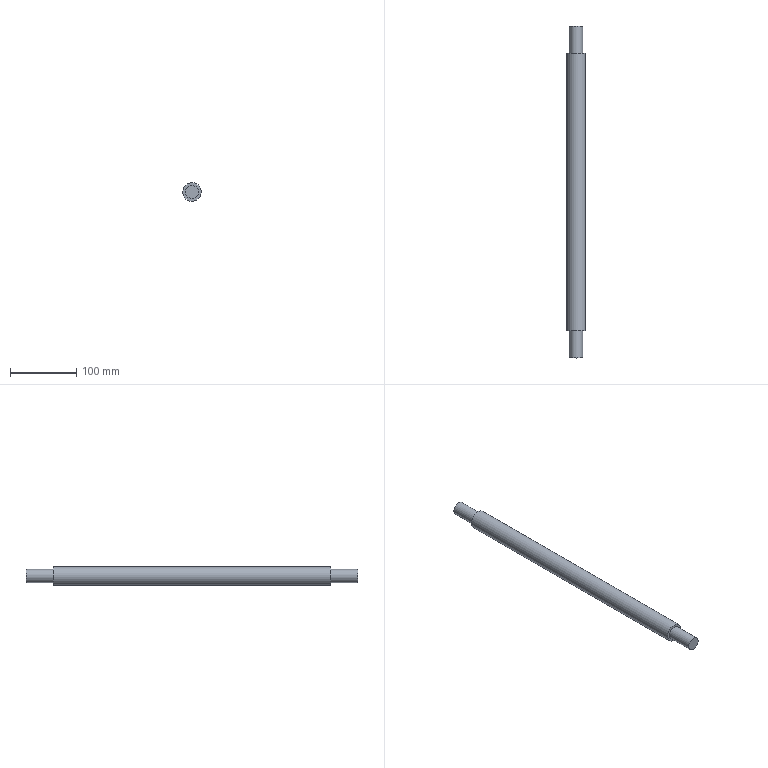Part | STEP file | SN10_002_010-03_EIXO | 1 solid | 7 faces | box 28 x 500.1 x 28 mm | volume 283207 mm3 | plane 4 | cylinder 3 | commonest cylinder face diameters 20 x2 28 x1
STEP:
#1=CARTESIAN_POINT('',(0.,0.,0.));
#2=DIRECTION('',(0.,0.,1.));
#3=DIRECTION('',(1.,0.,0.));
#4=AXIS2_PLACEMENT_3D('',#1,#2,#3);
#5=CARTESIAN_POINT('',(995.206,90.05,8.776));
#6=VERTEX_POINT('',#5);
#7=CARTESIAN_POINT('',(1000.,90.05,0.));
#8=DIRECTION('',(0.,-1.,0.));
#9=DIRECTION('',(1.,0.,0.));
#10=AXIS2_PLACEMENT_3D('',#7,#8,#9);
#11=CIRCLE('',#10,10.);
#12=CARTESIAN_POINT('',(1000.,-160.,0.));
#13=DIRECTION('',(0.,-1.,0.));
#14=DIRECTION('',(-0.4794,0.,0.8776));
#15=AXIS2_PLACEMENT_3D('',#12,#13,#14);
#16=CYLINDRICAL_SURFACE('',#15,10.);
#17=CARTESIAN_POINT('',(-2.071,-250.05));
#18=DIRECTION('',(1.,0.));
#19=VECTOR('',#18,1.);
#20=LINE('',#17,#19);
#21=(GEOMETRIC_REPRESENTATION_CONTEXT(2)PARAMETRIC_REPRESENTATION_CONTEXT()REPRESENTATION_CONTEXT('',''));
#22=DEFINITIONAL_REPRESENTATION('',(#20),#21);
#23=PCURVE('',#16,#22);
#24=CARTESIAN_POINT('',(1000.,90.05,10.));
#25=DIRECTION('',(0.,-1.,0.));
#26=DIRECTION('',(0.,0.,-1.));
#27=AXIS2_PLACEMENT_3D('',#24,#25,#26);
#28=PLANE('',#27);
#29=CARTESIAN_POINT('',(10.,0.));
#30=DIRECTION('',(0.,1.));
#31=AXIS2_PLACEMENT_2D('',#29,#30);
#32=CIRCLE('',#31,10.);
#33=(GEOMETRIC_REPRESENTATION_CONTEXT(2)PARAMETRIC_REPRESENTATION_CONTEXT()REPRESENTATION_CONTEXT('',''));
#34=DEFINITIONAL_REPRESENTATION('',(#32),#33);
#35=PCURVE('',#28,#34);
#36=SURFACE_CURVE('',#11,(#23,#35),.PCURVE_S1.);
#37=EDGE_CURVE('',#6,#6,#36,.T.);
#38=ORIENTED_EDGE('',*,*,#37,.T.);
#39=CARTESIAN_POINT('',(995.206,49.05,8.776));
#40=VERTEX_POINT('',#39);
#41=CARTESIAN_POINT('',(995.206,90.05,8.776));
#42=CARTESIAN_POINT('',(995.206,49.05,8.776));
#43=B_SPLINE_CURVE_WITH_KNOTS('',1,(#41,#42),.UNSPECIFIED.,.F.,.F.,(2,2),(-250.05,-209.05),.PIECEWISE_BEZIER_KNOTS.);
#44=CARTESIAN_POINT('',(6.283,0.));
#45=DIRECTION('',(0.,1.));
#46=VECTOR('',#45,1.);
#47=LINE('',#44,#46);
#48=(GEOMETRIC_REPRESENTATION_CONTEXT(2)PARAMETRIC_REPRESENTATION_CONTEXT()REPRESENTATION_CONTEXT('',''));
#49=DEFINITIONAL_REPRESENTATION('',(#47),#48);
#50=PCURVE('',#16,#49);
#51=CARTESIAN_POINT('',(0.,0.));
#52=DIRECTION('',(0.,1.));
#53=VECTOR('',#52,1.);
#54=LINE('',#51,#53);
#55=(GEOMETRIC_REPRESENTATION_CONTEXT(2)PARAMETRIC_REPRESENTATION_CONTEXT()REPRESENTATION_CONTEXT('',''));
#56=DEFINITIONAL_REPRESENTATION('',(#54),#55);
#57=PCURVE('',#16,#56);
#58=SEAM_CURVE('',#43,(#50,#57),.PCURVE_S1.);
#59=EDGE_CURVE('',#6,#40,#58,.T.);
#60=ORIENTED_EDGE('',*,*,#59,.T.);
#61=CARTESIAN_POINT('',(1000.,49.05,0.));
#62=DIRECTION('',(0.,-1.,0.));
#63=DIRECTION('',(1.,0.,0.));
#64=AXIS2_PLACEMENT_3D('',#61,#62,#63);
#65=CIRCLE('',#64,10.);
#66=CARTESIAN_POINT('',(-2.071,-209.05));
#67=DIRECTION('',(1.,0.));
#68=VECTOR('',#67,1.);
#69=LINE('',#66,#68);
#70=(GEOMETRIC_REPRESENTATION_CONTEXT(2)PARAMETRIC_REPRESENTATION_CONTEXT()REPRESENTATION_CONTEXT('',''));
#71=DEFINITIONAL_REPRESENTATION('',(#69),#70);
#72=PCURVE('',#16,#71);
#73=CARTESIAN_POINT('',(1000.,49.05,14.));
#74=DIRECTION('',(0.,-1.,0.));
#75=DIRECTION('',(0.,0.,-1.));
#76=AXIS2_PLACEMENT_3D('',#73,#74,#75);
#77=PLANE('',#76);
#78=CARTESIAN_POINT('',(14.,0.));
#79=DIRECTION('',(0.,1.));
#80=AXIS2_PLACEMENT_2D('',#78,#79);
#81=CIRCLE('',#80,10.);
#82=(GEOMETRIC_REPRESENTATION_CONTEXT(2)PARAMETRIC_REPRESENTATION_CONTEXT()REPRESENTATION_CONTEXT('',''));
#83=DEFINITIONAL_REPRESENTATION('',(#81),#82);
#84=PCURVE('',#77,#83);
#85=SURFACE_CURVE('',#65,(#72,#84),.PCURVE_S1.);
#86=EDGE_CURVE('',#40,#40,#85,.T.);
#87=ORIENTED_EDGE('',*,*,#86,.F.);
#88=ORIENTED_EDGE('',*,*,#59,.F.);
#89=EDGE_LOOP('',(#38,#60,#87,#88));
#90=FACE_BOUND('',#89,.T.);
#91=ADVANCED_FACE('',(#90),#16,.T.);
#92=CARTESIAN_POINT('',(993.288,49.05,12.286));
#93=VERTEX_POINT('',#92);
#94=CARTESIAN_POINT('',(1000.,49.05,0.));
#95=DIRECTION('',(0.,-1.,0.));
#96=DIRECTION('',(1.,0.,0.));
#97=AXIS2_PLACEMENT_3D('',#94,#95,#96);
#98=CIRCLE('',#97,14.);
#99=CARTESIAN_POINT('',(1000.,-160.,0.));
#100=DIRECTION('',(0.,-1.,0.));
#101=DIRECTION('',(-0.4794,0.,0.8776));
#102=AXIS2_PLACEMENT_3D('',#99,#100,#101);
#103=CYLINDRICAL_SURFACE('',#102,14.);
#104=CARTESIAN_POINT('',(-2.071,-209.05));
#105=DIRECTION('',(1.,0.));
#106=VECTOR('',#105,1.);
#107=LINE('',#104,#106);
#108=(GEOMETRIC_REPRESENTATION_CONTEXT(2)PARAMETRIC_REPRESENTATION_CONTEXT()REPRESENTATION_CONTEXT('',''));
#109=DEFINITIONAL_REPRESENTATION('',(#107),#108);
#110=PCURVE('',#103,#109);
#111=CARTESIAN_POINT('',(14.,0.));
#112=DIRECTION('',(0.,1.));
#113=AXIS2_PLACEMENT_2D('',#111,#112);
#114=CIRCLE('',#113,14.);
#115=(GEOMETRIC_REPRESENTATION_CONTEXT(2)PARAMETRIC_REPRESENTATION_CONTEXT()REPRESENTATION_CONTEXT('',''));
#116=DEFINITIONAL_REPRESENTATION('',(#114),#115);
#117=PCURVE('',#77,#116);
#118=SURFACE_CURVE('',#98,(#110,#117),.PCURVE_S1.);
#119=EDGE_CURVE('',#93,#93,#118,.T.);
#120=ORIENTED_EDGE('',*,*,#119,.T.);
#121=CARTESIAN_POINT('',(993.288,-369.05,12.286));
#122=VERTEX_POINT('',#121);
#123=CARTESIAN_POINT('',(993.288,49.05,12.286));
#124=CARTESIAN_POINT('',(993.288,-369.05,12.286));
#125=B_SPLINE_CURVE_WITH_KNOTS('',1,(#123,#124),.UNSPECIFIED.,.F.,.F.,(2,2),(-209.05,209.05),.PIECEWISE_BEZIER_KNOTS.);
#126=CARTESIAN_POINT('',(6.283,0.));
#127=DIRECTION('',(0.,1.));
#128=VECTOR('',#127,1.);
#129=LINE('',#126,#128);
#130=(GEOMETRIC_REPRESENTATION_CONTEXT(2)PARAMETRIC_REPRESENTATION_CONTEXT()REPRESENTATION_CONTEXT('',''));
#131=DEFINITIONAL_REPRESENTATION('',(#129),#130);
#132=PCURVE('',#103,#131);
#133=CARTESIAN_POINT('',(0.,0.));
#134=DIRECTION('',(0.,1.));
#135=VECTOR('',#134,1.);
#136=LINE('',#133,#135);
#137=(GEOMETRIC_REPRESENTATION_CONTEXT(2)PARAMETRIC_REPRESENTATION_CONTEXT()REPRESENTATION_CONTEXT('',''));
#138=DEFINITIONAL_REPRESENTATION('',(#136),#137);
#139=PCURVE('',#103,#138);
#140=SEAM_CURVE('',#125,(#132,#139),.PCURVE_S1.);
#141=EDGE_CURVE('',#93,#122,#140,.T.);
#142=ORIENTED_EDGE('',*,*,#141,.T.);
#143=CARTESIAN_POINT('',(1000.,-369.05,0.));
#144=DIRECTION('',(0.,-1.,0.));
#145=DIRECTION('',(1.,0.,0.));
#146=AXIS2_PLACEMENT_3D('',#143,#144,#145);
#147=CIRCLE('',#146,14.);
#148=CARTESIAN_POINT('',(-2.071,209.05));
#149=DIRECTION('',(1.,0.));
#150=VECTOR('',#149,1.);
#151=LINE('',#148,#150);
#152=(GEOMETRIC_REPRESENTATION_CONTEXT(2)PARAMETRIC_REPRESENTATION_CONTEXT()REPRESENTATION_CONTEXT('',''));
#153=DEFINITIONAL_REPRESENTATION('',(#151),#152);
#154=PCURVE('',#103,#153);
#155=CARTESIAN_POINT('',(1000.,-369.05,10.));
#156=DIRECTION('',(0.,-1.,0.));
#157=DIRECTION('',(0.,0.,-1.));
#158=AXIS2_PLACEMENT_3D('',#155,#156,#157);
#159=PLANE('',#158);
#160=CARTESIAN_POINT('',(10.,0.));
#161=DIRECTION('',(0.,1.));
#162=AXIS2_PLACEMENT_2D('',#160,#161);
#163=CIRCLE('',#162,14.);
#164=(GEOMETRIC_REPRESENTATION_CONTEXT(2)PARAMETRIC_REPRESENTATION_CONTEXT()REPRESENTATION_CONTEXT('',''));
#165=DEFINITIONAL_REPRESENTATION('',(#163),#164);
#166=PCURVE('',#159,#165);
#167=SURFACE_CURVE('',#147,(#154,#166),.PCURVE_S1.);
#168=EDGE_CURVE('',#122,#122,#167,.T.);
#169=ORIENTED_EDGE('',*,*,#168,.F.);
#170=ORIENTED_EDGE('',*,*,#141,.F.);
#171=EDGE_LOOP('',(#120,#142,#169,#170));
#172=FACE_BOUND('',#171,.T.);
#173=ADVANCED_FACE('',(#172),#103,.T.);
#174=CARTESIAN_POINT('',(995.206,-369.05,8.776));
#175=VERTEX_POINT('',#174);
#176=CARTESIAN_POINT('',(1000.,-369.05,0.));
#177=DIRECTION('',(0.,-1.,0.));
#178=DIRECTION('',(1.,0.,0.));
#179=AXIS2_PLACEMENT_3D('',#176,#177,#178);
#180=CIRCLE('',#179,10.);
#181=CARTESIAN_POINT('',(1000.,-160.,0.));
#182=DIRECTION('',(0.,-1.,0.));
#183=DIRECTION('',(-0.4794,0.,0.8776));
#184=AXIS2_PLACEMENT_3D('',#181,#182,#183);
#185=CYLINDRICAL_SURFACE('',#184,10.);
#186=CARTESIAN_POINT('',(-2.071,209.05));
#187=DIRECTION('',(1.,0.));
#188=VECTOR('',#187,1.);
#189=LINE('',#186,#188);
#190=(GEOMETRIC_REPRESENTATION_CONTEXT(2)PARAMETRIC_REPRESENTATION_CONTEXT()REPRESENTATION_CONTEXT('',''));
#191=DEFINITIONAL_REPRESENTATION('',(#189),#190);
#192=PCURVE('',#185,#191);
#193=CARTESIAN_POINT('',(10.,0.));
#194=DIRECTION('',(0.,1.));
#195=AXIS2_PLACEMENT_2D('',#193,#194);
#196=CIRCLE('',#195,10.);
#197=(GEOMETRIC_REPRESENTATION_CONTEXT(2)PARAMETRIC_REPRESENTATION_CONTEXT()REPRESENTATION_CONTEXT('',''));
#198=DEFINITIONAL_REPRESENTATION('',(#196),#197);
#199=PCURVE('',#159,#198);
#200=SURFACE_CURVE('',#180,(#192,#199),.PCURVE_S1.);
#201=EDGE_CURVE('',#175,#175,#200,.T.);
#202=ORIENTED_EDGE('',*,*,#201,.T.);
#203=CARTESIAN_POINT('',(995.206,-410.05,8.776));
#204=VERTEX_POINT('',#203);
#205=CARTESIAN_POINT('',(995.206,-369.05,8.776));
#206=CARTESIAN_POINT('',(995.206,-410.05,8.776));
#207=B_SPLINE_CURVE_WITH_KNOTS('',1,(#205,#206),.UNSPECIFIED.,.F.,.F.,(2,2),(209.05,250.05),.PIECEWISE_BEZIER_KNOTS.);
#208=CARTESIAN_POINT('',(6.283,0.));
#209=DIRECTION('',(0.,1.));
#210=VECTOR('',#209,1.);
#211=LINE('',#208,#210);
#212=(GEOMETRIC_REPRESENTATION_CONTEXT(2)PARAMETRIC_REPRESENTATION_CONTEXT()REPRESENTATION_CONTEXT('',''));
#213=DEFINITIONAL_REPRESENTATION('',(#211),#212);
#214=PCURVE('',#185,#213);
#215=CARTESIAN_POINT('',(0.,0.));
#216=DIRECTION('',(0.,1.));
#217=VECTOR('',#216,1.);
#218=LINE('',#215,#217);
#219=(GEOMETRIC_REPRESENTATION_CONTEXT(2)PARAMETRIC_REPRESENTATION_CONTEXT()REPRESENTATION_CONTEXT('',''));
#220=DEFINITIONAL_REPRESENTATION('',(#218),#219);
#221=PCURVE('',#185,#220);
#222=SEAM_CURVE('',#207,(#214,#221),.PCURVE_S1.);
#223=EDGE_CURVE('',#175,#204,#222,.T.);
#224=ORIENTED_EDGE('',*,*,#223,.T.);
#225=CARTESIAN_POINT('',(1000.,-410.05,0.));
#226=DIRECTION('',(0.,-1.,0.));
#227=DIRECTION('',(1.,0.,0.));
#228=AXIS2_PLACEMENT_3D('',#225,#226,#227);
#229=CIRCLE('',#228,10.);
#230=CARTESIAN_POINT('',(-2.071,250.05));
#231=DIRECTION('',(1.,0.));
#232=VECTOR('',#231,1.);
#233=LINE('',#230,#232);
#234=(GEOMETRIC_REPRESENTATION_CONTEXT(2)PARAMETRIC_REPRESENTATION_CONTEXT()REPRESENTATION_CONTEXT('',''));
#235=DEFINITIONAL_REPRESENTATION('',(#233),#234);
#236=PCURVE('',#185,#235);
#237=CARTESIAN_POINT('',(1000.,-410.05,0.));
#238=DIRECTION('',(0.,-1.,0.));
#239=DIRECTION('',(0.,0.,-1.));
#240=AXIS2_PLACEMENT_3D('',#237,#238,#239);
#241=PLANE('',#240);
#242=CARTESIAN_POINT('',(0.,0.));
#243=DIRECTION('',(0.,1.));
#244=AXIS2_PLACEMENT_2D('',#242,#243);
#245=CIRCLE('',#244,10.);
#246=(GEOMETRIC_REPRESENTATION_CONTEXT(2)PARAMETRIC_REPRESENTATION_CONTEXT()REPRESENTATION_CONTEXT('',''));
#247=DEFINITIONAL_REPRESENTATION('',(#245),#246);
#248=PCURVE('',#241,#247);
#249=SURFACE_CURVE('',#229,(#236,#248),.PCURVE_S1.);
#250=EDGE_CURVE('',#204,#204,#249,.T.);
#251=ORIENTED_EDGE('',*,*,#250,.F.);
#252=ORIENTED_EDGE('',*,*,#223,.F.);
#253=EDGE_LOOP('',(#202,#224,#251,#252));
#254=FACE_BOUND('',#253,.T.);
#255=ADVANCED_FACE('',(#254),#185,.T.);
#256=ORIENTED_EDGE('',*,*,#37,.F.);
#257=EDGE_LOOP('',(#256));
#258=FACE_BOUND('',#257,.T.);
#259=ADVANCED_FACE('',(#258),#28,.F.);
#260=ORIENTED_EDGE('',*,*,#119,.F.);
#261=EDGE_LOOP('',(#260));
#262=FACE_BOUND('',#261,.T.);
#263=ORIENTED_EDGE('',*,*,#86,.T.);
#264=EDGE_LOOP('',(#263));
#265=FACE_BOUND('',#264,.T.);
#266=ADVANCED_FACE('',(#262,#265),#77,.F.);
#267=ORIENTED_EDGE('',*,*,#168,.T.);
#268=EDGE_LOOP('',(#267));
#269=FACE_BOUND('',#268,.T.);
#270=ORIENTED_EDGE('',*,*,#201,.F.);
#271=EDGE_LOOP('',(#270));
#272=FACE_BOUND('',#271,.T.);
#273=ADVANCED_FACE('',(#269,#272),#159,.T.);
#274=ORIENTED_EDGE('',*,*,#250,.T.);
#275=EDGE_LOOP('',(#274));
#276=FACE_BOUND('',#275,.T.);
#277=ADVANCED_FACE('',(#276),#241,.T.);
#278=CLOSED_SHELL('',(#91,#173,#255,#259,#266,#273,#277));
#279=MANIFOLD_SOLID_BREP('',#278);
#280=(LENGTH_UNIT()NAMED_UNIT(*)SI_UNIT(.MILLI.,.METRE.));
#281=UNCERTAINTY_MEASURE_WITH_UNIT(LENGTH_MEASURE(0.00001),#280,'','');
#282=(NAMED_UNIT(*)PLANE_ANGLE_UNIT()SI_UNIT($,.RADIAN.));
#283=(NAMED_UNIT(*)SI_UNIT($,.STERADIAN.)SOLID_ANGLE_UNIT());
#284=(GEOMETRIC_REPRESENTATION_CONTEXT(3)GLOBAL_UNCERTAINTY_ASSIGNED_CONTEXT((#281))GLOBAL_UNIT_ASSIGNED_CONTEXT((#280,#282,#283))REPRESENTATION_CONTEXT('',''));
#285=ADVANCED_BREP_SHAPE_REPRESENTATION('',(#4,#279),#284);